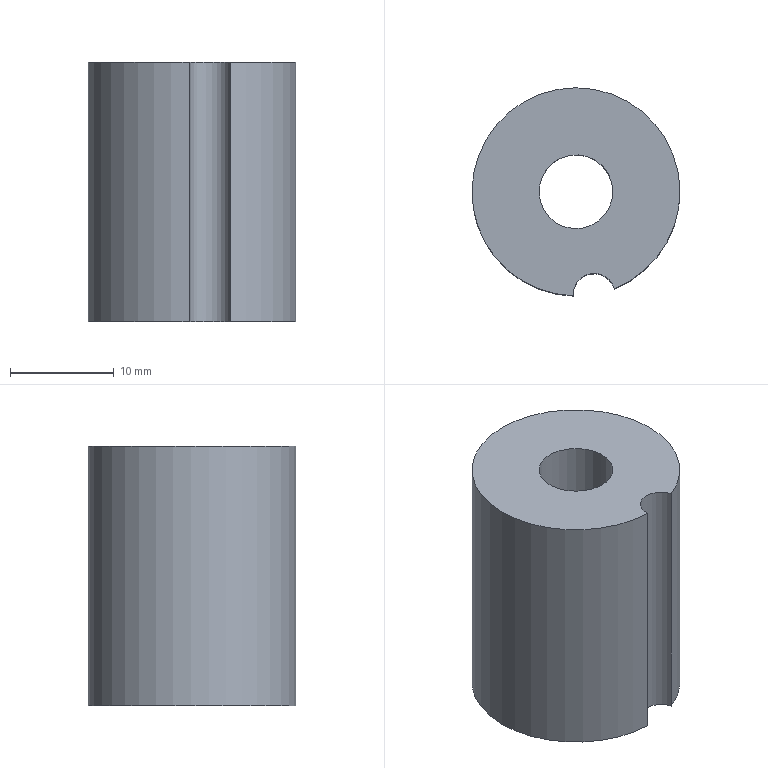Part | NX | features solid 2 | 1 solid | 7 faces | box 20 x 19.997 x 25 mm | volume 5267 mm3 | cylinder 4 | plane 3 | commonest cylinder face diameters 4 x1 7.1 x1 12.6 x1 20 x1
STEP:
#1=CARTESIAN_POINT('',(-228.339,427.02,31.));
#2=VERTEX_POINT('',#1);
#3=CARTESIAN_POINT('',(-228.339,427.02,56.));
#4=VERTEX_POINT('',#3);
#5=CARTESIAN_POINT('',(-228.339,427.02,43.5));
#6=DIRECTION('',(0.,0.,1.));
#7=VECTOR('',#6,1000.);
#8=LINE('',#5,#7);
#9=EDGE_CURVE('',#2,#4,#8,.T.);
#10=ORIENTED_EDGE('',*,*,#9,.F.);
#11=CARTESIAN_POINT('',(-232.258,426.329,31.));
#12=VERTEX_POINT('',#11);
#13=CARTESIAN_POINT('',(-232.,436.325,31.));
#14=DIRECTION('',(0.,0.,1.));
#15=DIRECTION('',(0.1736,-0.9848,0.));
#16=AXIS2_PLACEMENT_3D('',#13,#14,#15);
#17=CIRCLE('',#16,10.);
#18=EDGE_CURVE('',#2,#12,#17,.T.);
#19=ORIENTED_EDGE('',*,*,#18,.T.);
#20=CARTESIAN_POINT('',(-232.258,426.329,56.));
#21=VERTEX_POINT('',#20);
#22=CARTESIAN_POINT('',(-232.258,426.329,43.5));
#23=DIRECTION('',(0.,0.,1.));
#24=VECTOR('',#23,1000.);
#25=LINE('',#22,#24);
#26=EDGE_CURVE('',#21,#12,#25,.F.);
#27=ORIENTED_EDGE('',*,*,#26,.F.);
#28=CARTESIAN_POINT('',(-232.,436.325,56.));
#29=DIRECTION('',(0.,0.,1.));
#30=DIRECTION('',(0.1736,-0.9848,0.));
#31=AXIS2_PLACEMENT_3D('',#28,#29,#30);
#32=CIRCLE('',#31,10.);
#33=EDGE_CURVE('',#4,#21,#32,.T.);
#34=ORIENTED_EDGE('',*,*,#33,.F.);
#35=EDGE_LOOP('',(#10,#19,#27,#34));
#36=FACE_BOUND('',#35,.T.);
#37=CARTESIAN_POINT('',(-232.,436.325,31.));
#38=DIRECTION('',(0.,0.,1.));
#39=DIRECTION('',(0.1736,-0.9848,0.));
#40=AXIS2_PLACEMENT_3D('',#37,#38,#39);
#41=CYLINDRICAL_SURFACE('',#40,10.);
#42=ADVANCED_FACE('',(#36),#41,.T.);
#43=CARTESIAN_POINT('',(-230.906,430.121,31.));
#44=VERTEX_POINT('',#43);
#45=CARTESIAN_POINT('',(-232.,436.325,31.));
#46=DIRECTION('',(0.,0.,1.));
#47=DIRECTION('',(0.1736,-0.9848,0.));
#48=AXIS2_PLACEMENT_3D('',#45,#46,#47);
#49=CIRCLE('',#48,6.3);
#50=EDGE_CURVE('',#44,#44,#49,.T.);
#51=ORIENTED_EDGE('',*,*,#50,.T.);
#52=EDGE_LOOP('',(#51));
#53=FACE_BOUND('',#52,.T.);
#54=ORIENTED_EDGE('',*,*,#18,.F.);
#55=CARTESIAN_POINT('',(-230.264,426.477,31.));
#56=DIRECTION('',(0.,0.,1.));
#57=DIRECTION('',(0.1736,-0.9848,0.));
#58=AXIS2_PLACEMENT_3D('',#55,#56,#57);
#59=CIRCLE('',#58,2.);
#60=EDGE_CURVE('',#2,#12,#59,.T.);
#61=ORIENTED_EDGE('',*,*,#60,.T.);
#62=EDGE_LOOP('',(#54,#61));
#63=FACE_BOUND('',#62,.T.);
#64=CARTESIAN_POINT('',(-232.,436.325,31.));
#65=DIRECTION('',(0.,0.,1.));
#66=DIRECTION('',(0.1736,-0.9848,0.));
#67=AXIS2_PLACEMENT_3D('',#64,#65,#66);
#68=PLANE('',#67);
#69=ADVANCED_FACE('',(#53,#63),#68,.F.);
#70=CARTESIAN_POINT('',(-231.384,432.829,56.));
#71=VERTEX_POINT('',#70);
#72=CARTESIAN_POINT('',(-232.,436.325,56.));
#73=DIRECTION('',(0.,0.,1.));
#74=DIRECTION('',(0.1736,-0.9848,0.));
#75=AXIS2_PLACEMENT_3D('',#72,#73,#74);
#76=CIRCLE('',#75,3.55);
#77=EDGE_CURVE('',#71,#71,#76,.T.);
#78=ORIENTED_EDGE('',*,*,#77,.F.);
#79=EDGE_LOOP('',(#78));
#80=FACE_BOUND('',#79,.T.);
#81=CARTESIAN_POINT('',(-230.264,426.477,56.));
#82=DIRECTION('',(0.,0.,1.));
#83=DIRECTION('',(0.1736,-0.9848,0.));
#84=AXIS2_PLACEMENT_3D('',#81,#82,#83);
#85=CIRCLE('',#84,2.);
#86=EDGE_CURVE('',#4,#21,#85,.T.);
#87=ORIENTED_EDGE('',*,*,#86,.F.);
#88=ORIENTED_EDGE('',*,*,#33,.T.);
#89=EDGE_LOOP('',(#87,#88));
#90=FACE_BOUND('',#89,.T.);
#91=CARTESIAN_POINT('',(-232.,436.325,56.));
#92=DIRECTION('',(0.,0.,1.));
#93=DIRECTION('',(0.1736,-0.9848,0.));
#94=AXIS2_PLACEMENT_3D('',#91,#92,#93);
#95=PLANE('',#94);
#96=ADVANCED_FACE('',(#80,#90),#95,.T.);
#97=ORIENTED_EDGE('',*,*,#50,.F.);
#98=EDGE_LOOP('',(#97));
#99=FACE_BOUND('',#98,.T.);
#100=CARTESIAN_POINT('',(-230.906,430.121,48.));
#101=VERTEX_POINT('',#100);
#102=CARTESIAN_POINT('',(-232.,436.325,48.));
#103=DIRECTION('',(0.,0.,1.));
#104=DIRECTION('',(0.1736,-0.9848,0.));
#105=AXIS2_PLACEMENT_3D('',#102,#103,#104);
#106=CIRCLE('',#105,6.3);
#107=EDGE_CURVE('',#101,#101,#106,.T.);
#108=ORIENTED_EDGE('',*,*,#107,.T.);
#109=EDGE_LOOP('',(#108));
#110=FACE_BOUND('',#109,.T.);
#111=CARTESIAN_POINT('',(-232.,436.325,31.));
#112=DIRECTION('',(0.,0.,1.));
#113=DIRECTION('',(0.1736,-0.9848,0.));
#114=AXIS2_PLACEMENT_3D('',#111,#112,#113);
#115=CYLINDRICAL_SURFACE('',#114,6.3);
#116=ADVANCED_FACE('',(#99,#110),#115,.F.);
#117=CARTESIAN_POINT('',(-231.384,432.829,48.));
#118=VERTEX_POINT('',#117);
#119=CARTESIAN_POINT('',(-232.,436.325,48.));
#120=DIRECTION('',(0.,0.,1.));
#121=DIRECTION('',(0.1736,-0.9848,0.));
#122=AXIS2_PLACEMENT_3D('',#119,#120,#121);
#123=CIRCLE('',#122,3.55);
#124=EDGE_CURVE('',#118,#118,#123,.T.);
#125=ORIENTED_EDGE('',*,*,#124,.T.);
#126=EDGE_LOOP('',(#125));
#127=FACE_BOUND('',#126,.T.);
#128=ORIENTED_EDGE('',*,*,#107,.F.);
#129=EDGE_LOOP('',(#128));
#130=FACE_BOUND('',#129,.T.);
#131=CARTESIAN_POINT('',(-232.,436.325,48.));
#132=DIRECTION('',(0.,0.,1.));
#133=DIRECTION('',(0.1736,-0.9848,0.));
#134=AXIS2_PLACEMENT_3D('',#131,#132,#133);
#135=PLANE('',#134);
#136=ADVANCED_FACE('',(#127,#130),#135,.F.);
#137=ORIENTED_EDGE('',*,*,#9,.T.);
#138=ORIENTED_EDGE('',*,*,#86,.T.);
#139=ORIENTED_EDGE('',*,*,#26,.T.);
#140=ORIENTED_EDGE('',*,*,#60,.F.);
#141=EDGE_LOOP('',(#137,#138,#139,#140));
#142=FACE_BOUND('',#141,.T.);
#143=CARTESIAN_POINT('',(-230.264,426.477,31.));
#144=DIRECTION('',(0.,0.,1.));
#145=DIRECTION('',(0.1736,-0.9848,0.));
#146=AXIS2_PLACEMENT_3D('',#143,#144,#145);
#147=CYLINDRICAL_SURFACE('',#146,2.);
#148=ADVANCED_FACE('',(#142),#147,.F.);
#149=ORIENTED_EDGE('',*,*,#77,.T.);
#150=EDGE_LOOP('',(#149));
#151=FACE_BOUND('',#150,.T.);
#152=ORIENTED_EDGE('',*,*,#124,.F.);
#153=EDGE_LOOP('',(#152));
#154=FACE_BOUND('',#153,.T.);
#155=CARTESIAN_POINT('',(-232.,436.325,31.));
#156=DIRECTION('',(0.,0.,1.));
#157=DIRECTION('',(0.1736,-0.9848,0.));
#158=AXIS2_PLACEMENT_3D('',#155,#156,#157);
#159=CYLINDRICAL_SURFACE('',#158,3.55);
#160=ADVANCED_FACE('',(#151,#154),#159,.F.);
#161=CLOSED_SHELL('',(#42,#69,#96,#116,#136,#148,#160));
#162=MANIFOLD_SOLID_BREP('',#161);
#163=(LENGTH_UNIT()NAMED_UNIT(*)SI_UNIT(.MILLI.,.METRE.));
#164=UNCERTAINTY_MEASURE_WITH_UNIT(LENGTH_MEASURE(0.00001),#163,'','');
#165=(NAMED_UNIT(*)PLANE_ANGLE_UNIT()SI_UNIT($,.RADIAN.));
#166=(NAMED_UNIT(*)SI_UNIT($,.STERADIAN.)SOLID_ANGLE_UNIT());
#167=(GEOMETRIC_REPRESENTATION_CONTEXT(3)GLOBAL_UNCERTAINTY_ASSIGNED_CONTEXT((#164))GLOBAL_UNIT_ASSIGNED_CONTEXT((#163,#165,#166))REPRESENTATION_CONTEXT('',''));
#168=ADVANCED_BREP_SHAPE_REPRESENTATION('',(#162),#167);